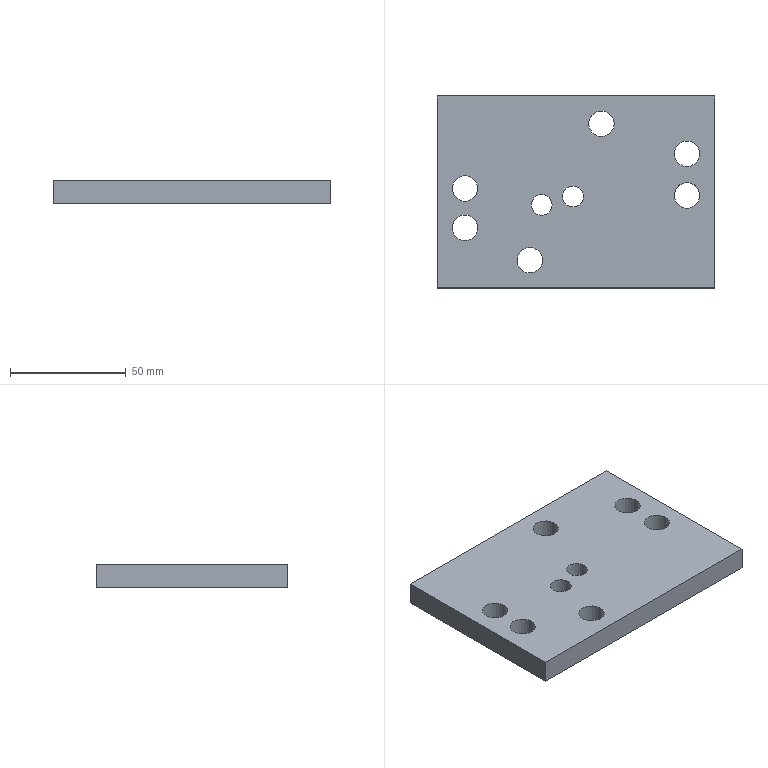Part | NX | features solid 2 | 1 solid | 14 faces | box 120 x 83 x 10 mm | volume 92626 mm3 | cylinder 8 | plane 6 | commonest cylinder face diameters 11 x6 9 x2
STEP:
#1=CARTESIAN_POINT('',(1379.835,54.431,78.));
#2=VERTEX_POINT('',#1);
#3=CARTESIAN_POINT('',(1384.335,54.431,78.));
#4=DIRECTION('',(0.,0.,-1.));
#5=DIRECTION('',(-1.,0.,0.));
#6=AXIS2_PLACEMENT_3D('',#3,#4,#5);
#7=CIRCLE('',#6,4.5);
#8=EDGE_CURVE('',#2,#2,#7,.F.);
#9=ORIENTED_EDGE('',*,*,#8,.F.);
#10=EDGE_LOOP('',(#9));
#11=FACE_BOUND('',#10,.T.);
#12=CARTESIAN_POINT('',(1379.835,54.431,88.));
#13=VERTEX_POINT('',#12);
#14=CARTESIAN_POINT('',(1384.335,54.431,88.));
#15=DIRECTION('',(0.,0.,-1.));
#16=DIRECTION('',(-1.,0.,0.));
#17=AXIS2_PLACEMENT_3D('',#14,#15,#16);
#18=CIRCLE('',#17,4.5);
#19=EDGE_CURVE('',#13,#13,#18,.F.);
#20=ORIENTED_EDGE('',*,*,#19,.T.);
#21=EDGE_LOOP('',(#20));
#22=FACE_BOUND('',#21,.T.);
#23=CARTESIAN_POINT('',(1384.335,54.431,78.));
#24=DIRECTION('',(0.,0.,-1.));
#25=DIRECTION('',(-1.,0.,0.));
#26=AXIS2_PLACEMENT_3D('',#23,#24,#25);
#27=CYLINDRICAL_SURFACE('',#26,4.5);
#28=ADVANCED_FACE('',(#11,#22),#27,.F.);
#29=CARTESIAN_POINT('',(1366.312,50.807,78.));
#30=VERTEX_POINT('',#29);
#31=CARTESIAN_POINT('',(1370.812,50.807,78.));
#32=DIRECTION('',(0.,0.,-1.));
#33=DIRECTION('',(-1.,0.,0.));
#34=AXIS2_PLACEMENT_3D('',#31,#32,#33);
#35=CIRCLE('',#34,4.5);
#36=EDGE_CURVE('',#30,#30,#35,.T.);
#37=ORIENTED_EDGE('',*,*,#36,.T.);
#38=EDGE_LOOP('',(#37));
#39=FACE_BOUND('',#38,.T.);
#40=CARTESIAN_POINT('',(1366.312,50.807,88.));
#41=VERTEX_POINT('',#40);
#42=CARTESIAN_POINT('',(1370.812,50.807,88.));
#43=DIRECTION('',(0.,0.,-1.));
#44=DIRECTION('',(-1.,0.,0.));
#45=AXIS2_PLACEMENT_3D('',#42,#43,#44);
#46=CIRCLE('',#45,4.5);
#47=EDGE_CURVE('',#41,#41,#46,.T.);
#48=ORIENTED_EDGE('',*,*,#47,.F.);
#49=EDGE_LOOP('',(#48));
#50=FACE_BOUND('',#49,.T.);
#51=CARTESIAN_POINT('',(1370.812,50.807,78.));
#52=DIRECTION('',(0.,0.,-1.));
#53=DIRECTION('',(-1.,0.,0.));
#54=AXIS2_PLACEMENT_3D('',#51,#52,#53);
#55=CYLINDRICAL_SURFACE('',#54,4.5);
#56=ADVANCED_FACE('',(#39,#50),#55,.F.);
#57=CARTESIAN_POINT('',(1325.653,97.891,88.));
#58=VERTEX_POINT('',#57);
#59=CARTESIAN_POINT('',(1325.653,97.891,78.));
#60=VERTEX_POINT('',#59);
#61=CARTESIAN_POINT('',(1325.653,97.891,78.));
#62=DIRECTION('',(0.,0.,1.));
#63=VECTOR('',#62,1000.);
#64=LINE('',#61,#63);
#65=EDGE_CURVE('',#58,#60,#64,.F.);
#66=ORIENTED_EDGE('',*,*,#65,.T.);
#67=CARTESIAN_POINT('',(1325.653,14.891,78.));
#68=VERTEX_POINT('',#67);
#69=CARTESIAN_POINT('',(1325.653,54.457,78.));
#70=DIRECTION('',(0.,-1.,0.));
#71=VECTOR('',#70,1000.);
#72=LINE('',#69,#71);
#73=EDGE_CURVE('',#68,#60,#72,.F.);
#74=ORIENTED_EDGE('',*,*,#73,.F.);
#75=CARTESIAN_POINT('',(1325.653,14.891,88.));
#76=VERTEX_POINT('',#75);
#77=CARTESIAN_POINT('',(1325.653,14.891,78.));
#78=DIRECTION('',(0.,0.,1.));
#79=VECTOR('',#78,1000.);
#80=LINE('',#77,#79);
#81=EDGE_CURVE('',#76,#68,#80,.F.);
#82=ORIENTED_EDGE('',*,*,#81,.F.);
#83=CARTESIAN_POINT('',(1325.653,0.000000688,88.));
#84=DIRECTION('',(0.,-1.,0.));
#85=VECTOR('',#84,1000.);
#86=LINE('',#83,#85);
#87=EDGE_CURVE('',#76,#58,#86,.F.);
#88=ORIENTED_EDGE('',*,*,#87,.T.);
#89=EDGE_LOOP('',(#66,#74,#82,#88));
#90=FACE_BOUND('',#89,.T.);
#91=CARTESIAN_POINT('',(1325.653,54.457,78.));
#92=DIRECTION('',(1.,0.,0.));
#93=DIRECTION('',(0.,-1.,0.));
#94=AXIS2_PLACEMENT_3D('',#91,#92,#93);
#95=PLANE('',#94);
#96=ADVANCED_FACE('',(#90),#95,.F.);
#97=CARTESIAN_POINT('',(1445.653,97.891,88.));
#98=VERTEX_POINT('',#97);
#99=CARTESIAN_POINT('',(1445.653,97.891,78.));
#100=VERTEX_POINT('',#99);
#101=CARTESIAN_POINT('',(1445.653,97.891,78.));
#102=DIRECTION('',(0.,0.,1.));
#103=VECTOR('',#102,1000.);
#104=LINE('',#101,#103);
#105=EDGE_CURVE('',#98,#100,#104,.F.);
#106=ORIENTED_EDGE('',*,*,#105,.T.);
#107=CARTESIAN_POINT('',(1387.005,97.891,78.));
#108=DIRECTION('',(-1.,0.,0.));
#109=VECTOR('',#108,1000.);
#110=LINE('',#107,#109);
#111=EDGE_CURVE('',#60,#100,#110,.F.);
#112=ORIENTED_EDGE('',*,*,#111,.F.);
#113=ORIENTED_EDGE('',*,*,#65,.F.);
#114=CARTESIAN_POINT('',(2186.158,97.891,88.));
#115=DIRECTION('',(1.,0.,0.));
#116=VECTOR('',#115,1000.);
#117=LINE('',#114,#116);
#118=EDGE_CURVE('',#58,#98,#117,.T.);
#119=ORIENTED_EDGE('',*,*,#118,.T.);
#120=EDGE_LOOP('',(#106,#112,#113,#119));
#121=FACE_BOUND('',#120,.T.);
#122=CARTESIAN_POINT('',(1387.005,97.891,78.));
#123=DIRECTION('',(0.,-1.,0.));
#124=DIRECTION('',(-1.,0.,0.));
#125=AXIS2_PLACEMENT_3D('',#122,#123,#124);
#126=PLANE('',#125);
#127=ADVANCED_FACE('',(#121),#126,.F.);
#128=CARTESIAN_POINT('',(1445.653,14.891,88.));
#129=VERTEX_POINT('',#128);
#130=CARTESIAN_POINT('',(1445.653,0.000000688,88.));
#131=DIRECTION('',(0.,-1.,0.));
#132=VECTOR('',#131,1000.);
#133=LINE('',#130,#132);
#134=EDGE_CURVE('',#98,#129,#133,.T.);
#135=ORIENTED_EDGE('',*,*,#134,.T.);
#136=CARTESIAN_POINT('',(1445.653,14.891,78.));
#137=VERTEX_POINT('',#136);
#138=CARTESIAN_POINT('',(1445.653,14.891,78.));
#139=DIRECTION('',(0.,0.,1.));
#140=VECTOR('',#139,1000.);
#141=LINE('',#138,#140);
#142=EDGE_CURVE('',#129,#137,#141,.F.);
#143=ORIENTED_EDGE('',*,*,#142,.T.);
#144=CARTESIAN_POINT('',(1445.653,54.457,78.));
#145=DIRECTION('',(0.,1.,0.));
#146=VECTOR('',#145,1000.);
#147=LINE('',#144,#146);
#148=EDGE_CURVE('',#100,#137,#147,.F.);
#149=ORIENTED_EDGE('',*,*,#148,.F.);
#150=ORIENTED_EDGE('',*,*,#105,.F.);
#151=EDGE_LOOP('',(#135,#143,#149,#150));
#152=FACE_BOUND('',#151,.T.);
#153=CARTESIAN_POINT('',(1445.653,54.457,78.));
#154=DIRECTION('',(-1.,0.,0.));
#155=DIRECTION('',(0.,1.,0.));
#156=AXIS2_PLACEMENT_3D('',#153,#154,#155);
#157=PLANE('',#156);
#158=ADVANCED_FACE('',(#152),#157,.F.);
#159=ORIENTED_EDGE('',*,*,#81,.T.);
#160=CARTESIAN_POINT('',(1387.005,14.891,78.));
#161=DIRECTION('',(1.,0.,0.));
#162=VECTOR('',#161,1000.);
#163=LINE('',#160,#162);
#164=EDGE_CURVE('',#137,#68,#163,.F.);
#165=ORIENTED_EDGE('',*,*,#164,.F.);
#166=ORIENTED_EDGE('',*,*,#142,.F.);
#167=CARTESIAN_POINT('',(2186.158,14.891,88.));
#168=DIRECTION('',(1.,0.,0.));
#169=VECTOR('',#168,1000.);
#170=LINE('',#167,#169);
#171=EDGE_CURVE('',#129,#76,#170,.F.);
#172=ORIENTED_EDGE('',*,*,#171,.T.);
#173=EDGE_LOOP('',(#159,#165,#166,#172));
#174=FACE_BOUND('',#173,.T.);
#175=CARTESIAN_POINT('',(1387.005,14.891,78.));
#176=DIRECTION('',(0.,1.,0.));
#177=DIRECTION('',(1.,0.,0.));
#178=AXIS2_PLACEMENT_3D('',#175,#176,#177);
#179=PLANE('',#178);
#180=ADVANCED_FACE('',(#174),#179,.F.);
#181=CARTESIAN_POINT('',(1360.153,26.891,78.));
#182=VERTEX_POINT('',#181);
#183=CARTESIAN_POINT('',(1365.653,26.891,78.));
#184=DIRECTION('',(0.,0.,-1.));
#185=DIRECTION('',(-1.,0.,0.));
#186=AXIS2_PLACEMENT_3D('',#183,#184,#185);
#187=CIRCLE('',#186,5.5);
#188=EDGE_CURVE('',#182,#182,#187,.F.);
#189=ORIENTED_EDGE('',*,*,#188,.F.);
#190=EDGE_LOOP('',(#189));
#191=FACE_BOUND('',#190,.T.);
#192=CARTESIAN_POINT('',(1360.153,26.891,88.));
#193=VERTEX_POINT('',#192);
#194=CARTESIAN_POINT('',(1365.653,26.891,88.));
#195=DIRECTION('',(0.,0.,-1.));
#196=DIRECTION('',(-1.,0.,0.));
#197=AXIS2_PLACEMENT_3D('',#194,#195,#196);
#198=CIRCLE('',#197,5.5);
#199=EDGE_CURVE('',#193,#193,#198,.F.);
#200=ORIENTED_EDGE('',*,*,#199,.T.);
#201=EDGE_LOOP('',(#200));
#202=FACE_BOUND('',#201,.T.);
#203=CARTESIAN_POINT('',(1365.653,26.891,78.));
#204=DIRECTION('',(0.,0.,-1.));
#205=DIRECTION('',(-1.,0.,0.));
#206=AXIS2_PLACEMENT_3D('',#203,#204,#205);
#207=CYLINDRICAL_SURFACE('',#206,5.5);
#208=ADVANCED_FACE('',(#191,#202),#207,.F.);
#209=CARTESIAN_POINT('',(1332.153,57.891,78.));
#210=VERTEX_POINT('',#209);
#211=CARTESIAN_POINT('',(1337.653,57.891,78.));
#212=DIRECTION('',(0.,0.,-1.));
#213=DIRECTION('',(-1.,0.,0.));
#214=AXIS2_PLACEMENT_3D('',#211,#212,#213);
#215=CIRCLE('',#214,5.5);
#216=EDGE_CURVE('',#210,#210,#215,.F.);
#217=ORIENTED_EDGE('',*,*,#216,.F.);
#218=EDGE_LOOP('',(#217));
#219=FACE_BOUND('',#218,.T.);
#220=CARTESIAN_POINT('',(1332.153,57.891,88.));
#221=VERTEX_POINT('',#220);
#222=CARTESIAN_POINT('',(1337.653,57.891,88.));
#223=DIRECTION('',(0.,0.,-1.));
#224=DIRECTION('',(-1.,0.,0.));
#225=AXIS2_PLACEMENT_3D('',#222,#223,#224);
#226=CIRCLE('',#225,5.5);
#227=EDGE_CURVE('',#221,#221,#226,.F.);
#228=ORIENTED_EDGE('',*,*,#227,.T.);
#229=EDGE_LOOP('',(#228));
#230=FACE_BOUND('',#229,.T.);
#231=CARTESIAN_POINT('',(1337.653,57.891,78.));
#232=DIRECTION('',(0.,0.,-1.));
#233=DIRECTION('',(-1.,0.,0.));
#234=AXIS2_PLACEMENT_3D('',#231,#232,#233);
#235=CYLINDRICAL_SURFACE('',#234,5.5);
#236=ADVANCED_FACE('',(#219,#230),#235,.F.);
#237=CARTESIAN_POINT('',(1391.153,85.891,78.));
#238=VERTEX_POINT('',#237);
#239=CARTESIAN_POINT('',(1396.653,85.891,78.));
#240=DIRECTION('',(0.,0.,-1.));
#241=DIRECTION('',(-1.,0.,0.));
#242=AXIS2_PLACEMENT_3D('',#239,#240,#241);
#243=CIRCLE('',#242,5.5);
#244=EDGE_CURVE('',#238,#238,#243,.F.);
#245=ORIENTED_EDGE('',*,*,#244,.F.);
#246=EDGE_LOOP('',(#245));
#247=FACE_BOUND('',#246,.T.);
#248=CARTESIAN_POINT('',(1391.153,85.891,88.));
#249=VERTEX_POINT('',#248);
#250=CARTESIAN_POINT('',(1396.653,85.891,88.));
#251=DIRECTION('',(0.,0.,-1.));
#252=DIRECTION('',(-1.,0.,0.));
#253=AXIS2_PLACEMENT_3D('',#250,#251,#252);
#254=CIRCLE('',#253,5.5);
#255=EDGE_CURVE('',#249,#249,#254,.F.);
#256=ORIENTED_EDGE('',*,*,#255,.T.);
#257=EDGE_LOOP('',(#256));
#258=FACE_BOUND('',#257,.T.);
#259=CARTESIAN_POINT('',(1396.653,85.891,78.));
#260=DIRECTION('',(0.,0.,-1.));
#261=DIRECTION('',(-1.,0.,0.));
#262=AXIS2_PLACEMENT_3D('',#259,#260,#261);
#263=CYLINDRICAL_SURFACE('',#262,5.5);
#264=ADVANCED_FACE('',(#247,#258),#263,.F.);
#265=CARTESIAN_POINT('',(1428.153,54.891,78.));
#266=VERTEX_POINT('',#265);
#267=CARTESIAN_POINT('',(1433.653,54.891,78.));
#268=DIRECTION('',(0.,0.,-1.));
#269=DIRECTION('',(-1.,0.,0.));
#270=AXIS2_PLACEMENT_3D('',#267,#268,#269);
#271=CIRCLE('',#270,5.5);
#272=EDGE_CURVE('',#266,#266,#271,.F.);
#273=ORIENTED_EDGE('',*,*,#272,.F.);
#274=EDGE_LOOP('',(#273));
#275=FACE_BOUND('',#274,.T.);
#276=CARTESIAN_POINT('',(1428.153,54.891,88.));
#277=VERTEX_POINT('',#276);
#278=CARTESIAN_POINT('',(1433.653,54.891,88.));
#279=DIRECTION('',(0.,0.,-1.));
#280=DIRECTION('',(-1.,0.,0.));
#281=AXIS2_PLACEMENT_3D('',#278,#279,#280);
#282=CIRCLE('',#281,5.5);
#283=EDGE_CURVE('',#277,#277,#282,.F.);
#284=ORIENTED_EDGE('',*,*,#283,.T.);
#285=EDGE_LOOP('',(#284));
#286=FACE_BOUND('',#285,.T.);
#287=CARTESIAN_POINT('',(1433.653,54.891,78.));
#288=DIRECTION('',(0.,0.,-1.));
#289=DIRECTION('',(-1.,0.,0.));
#290=AXIS2_PLACEMENT_3D('',#287,#288,#289);
#291=CYLINDRICAL_SURFACE('',#290,5.5);
#292=ADVANCED_FACE('',(#275,#286),#291,.F.);
#293=CARTESIAN_POINT('',(1332.153,40.891,78.));
#294=VERTEX_POINT('',#293);
#295=CARTESIAN_POINT('',(1337.653,40.891,78.));
#296=DIRECTION('',(0.,0.,-1.));
#297=DIRECTION('',(-1.,0.,0.));
#298=AXIS2_PLACEMENT_3D('',#295,#296,#297);
#299=CIRCLE('',#298,5.5);
#300=EDGE_CURVE('',#294,#294,#299,.F.);
#301=ORIENTED_EDGE('',*,*,#300,.F.);
#302=EDGE_LOOP('',(#301));
#303=FACE_BOUND('',#302,.T.);
#304=CARTESIAN_POINT('',(1332.153,40.891,88.));
#305=VERTEX_POINT('',#304);
#306=CARTESIAN_POINT('',(1337.653,40.891,88.));
#307=DIRECTION('',(0.,0.,-1.));
#308=DIRECTION('',(-1.,0.,0.));
#309=AXIS2_PLACEMENT_3D('',#306,#307,#308);
#310=CIRCLE('',#309,5.5);
#311=EDGE_CURVE('',#305,#305,#310,.F.);
#312=ORIENTED_EDGE('',*,*,#311,.T.);
#313=EDGE_LOOP('',(#312));
#314=FACE_BOUND('',#313,.T.);
#315=CARTESIAN_POINT('',(1337.653,40.891,78.));
#316=DIRECTION('',(0.,0.,-1.));
#317=DIRECTION('',(-1.,0.,0.));
#318=AXIS2_PLACEMENT_3D('',#315,#316,#317);
#319=CYLINDRICAL_SURFACE('',#318,5.5);
#320=ADVANCED_FACE('',(#303,#314),#319,.F.);
#321=CARTESIAN_POINT('',(1428.153,72.891,78.));
#322=VERTEX_POINT('',#321);
#323=CARTESIAN_POINT('',(1433.653,72.891,78.));
#324=DIRECTION('',(0.,0.,-1.));
#325=DIRECTION('',(-1.,0.,0.));
#326=AXIS2_PLACEMENT_3D('',#323,#324,#325);
#327=CIRCLE('',#326,5.5);
#328=EDGE_CURVE('',#322,#322,#327,.F.);
#329=ORIENTED_EDGE('',*,*,#328,.F.);
#330=EDGE_LOOP('',(#329));
#331=FACE_BOUND('',#330,.T.);
#332=CARTESIAN_POINT('',(1428.153,72.891,88.));
#333=VERTEX_POINT('',#332);
#334=CARTESIAN_POINT('',(1433.653,72.891,88.));
#335=DIRECTION('',(0.,0.,-1.));
#336=DIRECTION('',(-1.,0.,0.));
#337=AXIS2_PLACEMENT_3D('',#334,#335,#336);
#338=CIRCLE('',#337,5.5);
#339=EDGE_CURVE('',#333,#333,#338,.F.);
#340=ORIENTED_EDGE('',*,*,#339,.T.);
#341=EDGE_LOOP('',(#340));
#342=FACE_BOUND('',#341,.T.);
#343=CARTESIAN_POINT('',(1433.653,72.891,78.));
#344=DIRECTION('',(0.,0.,-1.));
#345=DIRECTION('',(-1.,0.,0.));
#346=AXIS2_PLACEMENT_3D('',#343,#344,#345);
#347=CYLINDRICAL_SURFACE('',#346,5.5);
#348=ADVANCED_FACE('',(#331,#342),#347,.F.);
#349=ORIENTED_EDGE('',*,*,#19,.F.);
#350=EDGE_LOOP('',(#349));
#351=FACE_BOUND('',#350,.T.);
#352=ORIENTED_EDGE('',*,*,#339,.F.);
#353=EDGE_LOOP('',(#352));
#354=FACE_BOUND('',#353,.T.);
#355=ORIENTED_EDGE('',*,*,#311,.F.);
#356=EDGE_LOOP('',(#355));
#357=FACE_BOUND('',#356,.T.);
#358=ORIENTED_EDGE('',*,*,#283,.F.);
#359=EDGE_LOOP('',(#358));
#360=FACE_BOUND('',#359,.T.);
#361=ORIENTED_EDGE('',*,*,#255,.F.);
#362=EDGE_LOOP('',(#361));
#363=FACE_BOUND('',#362,.T.);
#364=ORIENTED_EDGE('',*,*,#227,.F.);
#365=EDGE_LOOP('',(#364));
#366=FACE_BOUND('',#365,.T.);
#367=ORIENTED_EDGE('',*,*,#199,.F.);
#368=EDGE_LOOP('',(#367));
#369=FACE_BOUND('',#368,.T.);
#370=ORIENTED_EDGE('',*,*,#171,.F.);
#371=ORIENTED_EDGE('',*,*,#134,.F.);
#372=ORIENTED_EDGE('',*,*,#118,.F.);
#373=ORIENTED_EDGE('',*,*,#87,.F.);
#374=EDGE_LOOP('',(#370,#371,#372,#373));
#375=FACE_BOUND('',#374,.T.);
#376=ORIENTED_EDGE('',*,*,#47,.T.);
#377=EDGE_LOOP('',(#376));
#378=FACE_BOUND('',#377,.T.);
#379=CARTESIAN_POINT('',(2186.158,0.000000688,88.));
#380=DIRECTION('',(0.,0.,-1.));
#381=DIRECTION('',(1.,0.,0.));
#382=AXIS2_PLACEMENT_3D('',#379,#380,#381);
#383=PLANE('',#382);
#384=ADVANCED_FACE('',(#351,#354,#357,#360,#363,#366,#369,#375,#378),#383,.F.);
#385=ORIENTED_EDGE('',*,*,#8,.T.);
#386=EDGE_LOOP('',(#385));
#387=FACE_BOUND('',#386,.T.);
#388=ORIENTED_EDGE('',*,*,#328,.T.);
#389=EDGE_LOOP('',(#388));
#390=FACE_BOUND('',#389,.T.);
#391=ORIENTED_EDGE('',*,*,#300,.T.);
#392=EDGE_LOOP('',(#391));
#393=FACE_BOUND('',#392,.T.);
#394=ORIENTED_EDGE('',*,*,#272,.T.);
#395=EDGE_LOOP('',(#394));
#396=FACE_BOUND('',#395,.T.);
#397=ORIENTED_EDGE('',*,*,#244,.T.);
#398=EDGE_LOOP('',(#397));
#399=FACE_BOUND('',#398,.T.);
#400=ORIENTED_EDGE('',*,*,#216,.T.);
#401=EDGE_LOOP('',(#400));
#402=FACE_BOUND('',#401,.T.);
#403=ORIENTED_EDGE('',*,*,#188,.T.);
#404=EDGE_LOOP('',(#403));
#405=FACE_BOUND('',#404,.T.);
#406=ORIENTED_EDGE('',*,*,#164,.T.);
#407=ORIENTED_EDGE('',*,*,#73,.T.);
#408=ORIENTED_EDGE('',*,*,#111,.T.);
#409=ORIENTED_EDGE('',*,*,#148,.T.);
#410=EDGE_LOOP('',(#406,#407,#408,#409));
#411=FACE_BOUND('',#410,.T.);
#412=ORIENTED_EDGE('',*,*,#36,.F.);
#413=EDGE_LOOP('',(#412));
#414=FACE_BOUND('',#413,.T.);
#415=CARTESIAN_POINT('',(2186.158,0.000000688,78.));
#416=DIRECTION('',(0.,0.,-1.));
#417=DIRECTION('',(1.,0.,0.));
#418=AXIS2_PLACEMENT_3D('',#415,#416,#417);
#419=PLANE('',#418);
#420=ADVANCED_FACE('',(#387,#390,#393,#396,#399,#402,#405,#411,#414),#419,.T.);
#421=CLOSED_SHELL('',(#28,#56,#96,#127,#158,#180,#208,#236,#264,#292,#320,#348,#384,#420));
#422=MANIFOLD_SOLID_BREP('',#421);
#423=(LENGTH_UNIT()NAMED_UNIT(*)SI_UNIT(.MILLI.,.METRE.));
#424=UNCERTAINTY_MEASURE_WITH_UNIT(LENGTH_MEASURE(0.00001),#423,'','');
#425=(NAMED_UNIT(*)PLANE_ANGLE_UNIT()SI_UNIT($,.RADIAN.));
#426=(NAMED_UNIT(*)SI_UNIT($,.STERADIAN.)SOLID_ANGLE_UNIT());
#427=(GEOMETRIC_REPRESENTATION_CONTEXT(3)GLOBAL_UNCERTAINTY_ASSIGNED_CONTEXT((#424))GLOBAL_UNIT_ASSIGNED_CONTEXT((#423,#425,#426))REPRESENTATION_CONTEXT('',''));
#428=ADVANCED_BREP_SHAPE_REPRESENTATION('',(#422),#427);